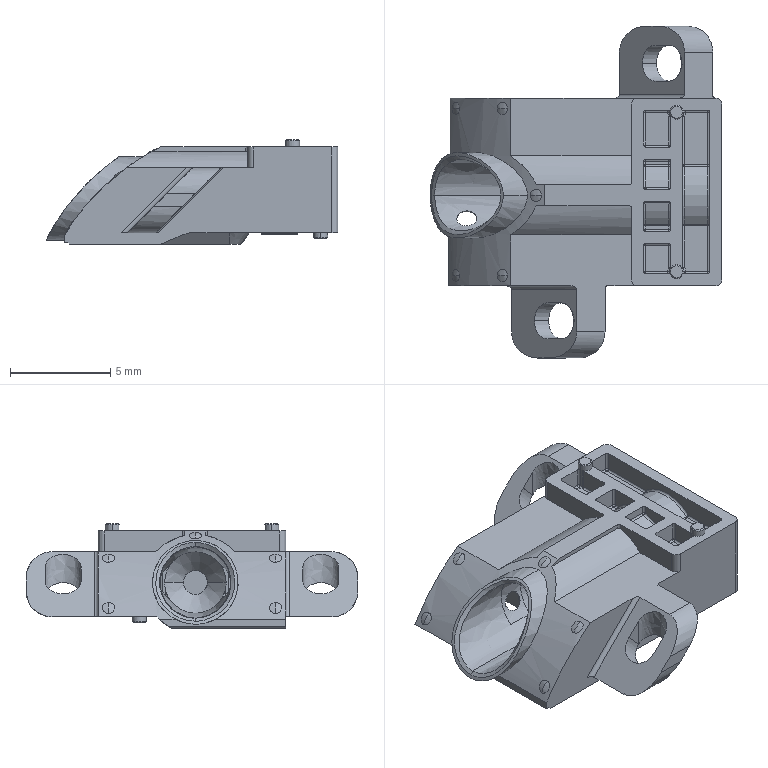Part | NX | 1 solid | 555 faces | box 14.541 x 16.558 x 5.218 mm | volume 281.084 mm3 | plane 260 | cylinder 181 | sphere 48 | torus 30 | cone 18 | spline 18 | commonest cylinder face diameters 0.2 x98 1 x14 0.4 x12 0.7 x8 0.6 x6 1.8 x6